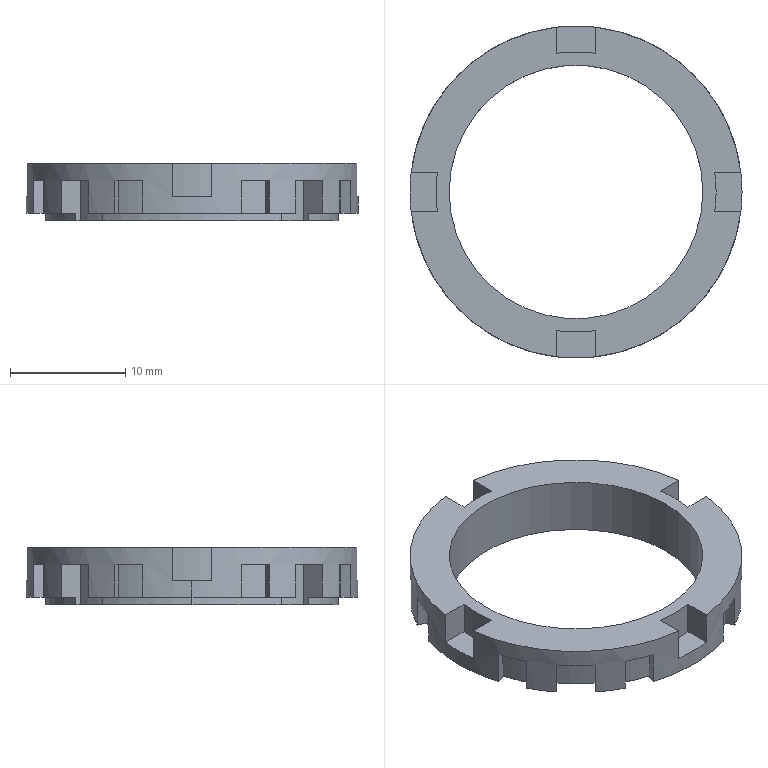Part | STEP file | A22NZ-A-403 | 1 solid | 80 faces | box 28.8 x 28.8 x 5 mm | volume 1033 mm3 | plane 54 | cylinder 26 | commonest cylinder face diameters 27 x8 24.3 x5 25.4 x5 24.36 x4 22 x2 28.8 x2